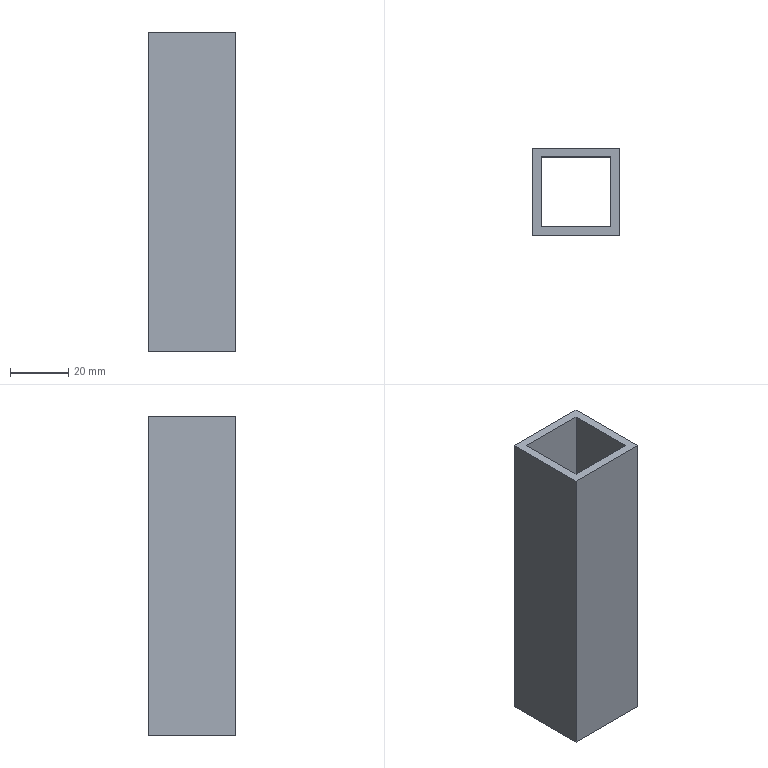Part | SolidWorks | features Cut 1, Extrusion 1 | 1 solid | 10 faces | box 30 x 30 x 110 mm | volume 35640 mm3 | plane 10
STEP:
#1=CARTESIAN_POINT('',(30.,0.,40.));
#2=VERTEX_POINT('',#1);
#3=CARTESIAN_POINT('',(0.,0.,40.));
#4=VERTEX_POINT('',#3);
#5=CARTESIAN_POINT('',(30.,0.,40.));
#6=DIRECTION('',(-1.,0.,0.));
#7=VECTOR('',#6,1000.);
#8=LINE('',#5,#7);
#9=EDGE_CURVE('',#2,#4,#8,.T.);
#10=ORIENTED_EDGE('',*,*,#9,.F.);
#11=CARTESIAN_POINT('',(30.,0.,150.));
#12=VERTEX_POINT('',#11);
#13=CARTESIAN_POINT('',(30.,0.,150.));
#14=DIRECTION('',(0.,0.,-1.));
#15=VECTOR('',#14,1000.);
#16=LINE('',#13,#15);
#17=EDGE_CURVE('',#12,#2,#16,.T.);
#18=ORIENTED_EDGE('',*,*,#17,.F.);
#19=CARTESIAN_POINT('',(0.,0.,150.));
#20=VERTEX_POINT('',#19);
#21=CARTESIAN_POINT('',(30.,0.,150.));
#22=DIRECTION('',(1.,0.,0.));
#23=VECTOR('',#22,1000.);
#24=LINE('',#21,#23);
#25=EDGE_CURVE('',#20,#12,#24,.T.);
#26=ORIENTED_EDGE('',*,*,#25,.F.);
#27=CARTESIAN_POINT('',(0.,0.,150.));
#28=DIRECTION('',(0.,0.,-1.));
#29=VECTOR('',#28,1000.);
#30=LINE('',#27,#29);
#31=EDGE_CURVE('',#20,#4,#30,.T.);
#32=ORIENTED_EDGE('',*,*,#31,.T.);
#33=EDGE_LOOP('',(#10,#18,#26,#32));
#34=FACE_OUTER_BOUND('',#33,.T.);
#35=CARTESIAN_POINT('',(30.,0.,150.));
#36=DIRECTION('',(0.,1.,0.));
#37=DIRECTION('',(0.,0.,1.));
#38=AXIS2_PLACEMENT_3D('',#35,#36,#37);
#39=PLANE('',#38);
#40=ADVANCED_FACE('',(#34),#39,.F.);
#41=CARTESIAN_POINT('',(30.,30.,40.));
#42=VERTEX_POINT('',#41);
#43=CARTESIAN_POINT('',(30.,30.,40.));
#44=DIRECTION('',(0.,-1.,0.));
#45=VECTOR('',#44,1000.);
#46=LINE('',#43,#45);
#47=EDGE_CURVE('',#42,#2,#46,.T.);
#48=ORIENTED_EDGE('',*,*,#47,.F.);
#49=CARTESIAN_POINT('',(30.,30.,150.));
#50=VERTEX_POINT('',#49);
#51=CARTESIAN_POINT('',(30.,30.,150.));
#52=DIRECTION('',(0.,0.,-1.));
#53=VECTOR('',#52,1000.);
#54=LINE('',#51,#53);
#55=EDGE_CURVE('',#50,#42,#54,.T.);
#56=ORIENTED_EDGE('',*,*,#55,.F.);
#57=CARTESIAN_POINT('',(30.,30.,150.));
#58=DIRECTION('',(0.,1.,0.));
#59=VECTOR('',#58,1000.);
#60=LINE('',#57,#59);
#61=EDGE_CURVE('',#12,#50,#60,.T.);
#62=ORIENTED_EDGE('',*,*,#61,.F.);
#63=ORIENTED_EDGE('',*,*,#17,.T.);
#64=EDGE_LOOP('',(#48,#56,#62,#63));
#65=FACE_OUTER_BOUND('',#64,.T.);
#66=CARTESIAN_POINT('',(30.,30.,150.));
#67=DIRECTION('',(-1.,0.,0.));
#68=DIRECTION('',(0.,0.,1.));
#69=AXIS2_PLACEMENT_3D('',#66,#67,#68);
#70=PLANE('',#69);
#71=ADVANCED_FACE('',(#65),#70,.F.);
#72=CARTESIAN_POINT('',(0.,30.,40.));
#73=VERTEX_POINT('',#72);
#74=CARTESIAN_POINT('',(0.,30.,40.));
#75=DIRECTION('',(1.,0.,0.));
#76=VECTOR('',#75,1000.);
#77=LINE('',#74,#76);
#78=EDGE_CURVE('',#73,#42,#77,.T.);
#79=ORIENTED_EDGE('',*,*,#78,.F.);
#80=CARTESIAN_POINT('',(0.,30.,150.));
#81=VERTEX_POINT('',#80);
#82=CARTESIAN_POINT('',(0.,30.,150.));
#83=DIRECTION('',(0.,0.,-1.));
#84=VECTOR('',#83,1000.);
#85=LINE('',#82,#84);
#86=EDGE_CURVE('',#81,#73,#85,.T.);
#87=ORIENTED_EDGE('',*,*,#86,.F.);
#88=CARTESIAN_POINT('',(0.,30.,150.));
#89=DIRECTION('',(-1.,0.,0.));
#90=VECTOR('',#89,1000.);
#91=LINE('',#88,#90);
#92=EDGE_CURVE('',#50,#81,#91,.T.);
#93=ORIENTED_EDGE('',*,*,#92,.F.);
#94=ORIENTED_EDGE('',*,*,#55,.T.);
#95=EDGE_LOOP('',(#79,#87,#93,#94));
#96=FACE_OUTER_BOUND('',#95,.T.);
#97=CARTESIAN_POINT('',(0.,30.,150.));
#98=DIRECTION('',(0.,-1.,0.));
#99=DIRECTION('',(0.,0.,-1.));
#100=AXIS2_PLACEMENT_3D('',#97,#98,#99);
#101=PLANE('',#100);
#102=ADVANCED_FACE('',(#96),#101,.F.);
#103=CARTESIAN_POINT('',(0.,0.,40.));
#104=DIRECTION('',(0.,1.,0.));
#105=VECTOR('',#104,1000.);
#106=LINE('',#103,#105);
#107=EDGE_CURVE('',#4,#73,#106,.T.);
#108=ORIENTED_EDGE('',*,*,#107,.F.);
#109=ORIENTED_EDGE('',*,*,#31,.F.);
#110=CARTESIAN_POINT('',(0.,0.,150.));
#111=DIRECTION('',(0.,-1.,0.));
#112=VECTOR('',#111,1000.);
#113=LINE('',#110,#112);
#114=EDGE_CURVE('',#81,#20,#113,.T.);
#115=ORIENTED_EDGE('',*,*,#114,.F.);
#116=ORIENTED_EDGE('',*,*,#86,.T.);
#117=EDGE_LOOP('',(#108,#109,#115,#116));
#118=FACE_OUTER_BOUND('',#117,.T.);
#119=CARTESIAN_POINT('',(0.,0.,150.));
#120=DIRECTION('',(1.,0.,0.));
#121=DIRECTION('',(0.,0.,-1.));
#122=AXIS2_PLACEMENT_3D('',#119,#120,#121);
#123=PLANE('',#122);
#124=ADVANCED_FACE('',(#118),#123,.F.);
#125=CARTESIAN_POINT('',(27.,3.,150.));
#126=VERTEX_POINT('',#125);
#127=CARTESIAN_POINT('',(27.,3.,40.));
#128=VERTEX_POINT('',#127);
#129=CARTESIAN_POINT('',(27.,3.,150.));
#130=DIRECTION('',(0.,0.,-1.));
#131=VECTOR('',#130,1000.);
#132=LINE('',#129,#131);
#133=EDGE_CURVE('',#126,#128,#132,.T.);
#134=ORIENTED_EDGE('',*,*,#133,.T.);
#135=CARTESIAN_POINT('',(3.,3.,40.));
#136=VERTEX_POINT('',#135);
#137=CARTESIAN_POINT('',(27.,3.,40.));
#138=DIRECTION('',(-1.,0.,0.));
#139=VECTOR('',#138,1000.);
#140=LINE('',#137,#139);
#141=EDGE_CURVE('',#128,#136,#140,.T.);
#142=ORIENTED_EDGE('',*,*,#141,.T.);
#143=CARTESIAN_POINT('',(3.,3.,150.));
#144=VERTEX_POINT('',#143);
#145=CARTESIAN_POINT('',(3.,3.,150.));
#146=DIRECTION('',(0.,0.,-1.));
#147=VECTOR('',#146,1000.);
#148=LINE('',#145,#147);
#149=EDGE_CURVE('',#144,#136,#148,.T.);
#150=ORIENTED_EDGE('',*,*,#149,.F.);
#151=CARTESIAN_POINT('',(27.,3.,150.));
#152=DIRECTION('',(1.,0.,0.));
#153=VECTOR('',#152,1000.);
#154=LINE('',#151,#153);
#155=EDGE_CURVE('',#144,#126,#154,.T.);
#156=ORIENTED_EDGE('',*,*,#155,.T.);
#157=EDGE_LOOP('',(#134,#142,#150,#156));
#158=FACE_OUTER_BOUND('',#157,.T.);
#159=CARTESIAN_POINT('',(27.,3.,150.));
#160=DIRECTION('',(0.,1.,0.));
#161=DIRECTION('',(0.,0.,1.));
#162=AXIS2_PLACEMENT_3D('',#159,#160,#161);
#163=PLANE('',#162);
#164=ADVANCED_FACE('',(#158),#163,.T.);
#165=CARTESIAN_POINT('',(27.,27.,150.));
#166=VERTEX_POINT('',#165);
#167=CARTESIAN_POINT('',(27.,27.,40.));
#168=VERTEX_POINT('',#167);
#169=CARTESIAN_POINT('',(27.,27.,150.));
#170=DIRECTION('',(0.,0.,-1.));
#171=VECTOR('',#170,1000.);
#172=LINE('',#169,#171);
#173=EDGE_CURVE('',#166,#168,#172,.T.);
#174=ORIENTED_EDGE('',*,*,#173,.T.);
#175=CARTESIAN_POINT('',(27.,27.,40.));
#176=DIRECTION('',(0.,-1.,0.));
#177=VECTOR('',#176,1000.);
#178=LINE('',#175,#177);
#179=EDGE_CURVE('',#168,#128,#178,.T.);
#180=ORIENTED_EDGE('',*,*,#179,.T.);
#181=ORIENTED_EDGE('',*,*,#133,.F.);
#182=CARTESIAN_POINT('',(27.,27.,150.));
#183=DIRECTION('',(0.,1.,0.));
#184=VECTOR('',#183,1000.);
#185=LINE('',#182,#184);
#186=EDGE_CURVE('',#126,#166,#185,.T.);
#187=ORIENTED_EDGE('',*,*,#186,.T.);
#188=EDGE_LOOP('',(#174,#180,#181,#187));
#189=FACE_OUTER_BOUND('',#188,.T.);
#190=CARTESIAN_POINT('',(27.,27.,150.));
#191=DIRECTION('',(-1.,0.,0.));
#192=DIRECTION('',(0.,0.,1.));
#193=AXIS2_PLACEMENT_3D('',#190,#191,#192);
#194=PLANE('',#193);
#195=ADVANCED_FACE('',(#189),#194,.T.);
#196=CARTESIAN_POINT('',(3.,27.,150.));
#197=VERTEX_POINT('',#196);
#198=CARTESIAN_POINT('',(3.,27.,40.));
#199=VERTEX_POINT('',#198);
#200=CARTESIAN_POINT('',(3.,27.,150.));
#201=DIRECTION('',(0.,0.,-1.));
#202=VECTOR('',#201,1000.);
#203=LINE('',#200,#202);
#204=EDGE_CURVE('',#197,#199,#203,.T.);
#205=ORIENTED_EDGE('',*,*,#204,.T.);
#206=CARTESIAN_POINT('',(3.,27.,40.));
#207=DIRECTION('',(1.,0.,0.));
#208=VECTOR('',#207,1000.);
#209=LINE('',#206,#208);
#210=EDGE_CURVE('',#199,#168,#209,.T.);
#211=ORIENTED_EDGE('',*,*,#210,.T.);
#212=ORIENTED_EDGE('',*,*,#173,.F.);
#213=CARTESIAN_POINT('',(3.,27.,150.));
#214=DIRECTION('',(-1.,0.,0.));
#215=VECTOR('',#214,1000.);
#216=LINE('',#213,#215);
#217=EDGE_CURVE('',#166,#197,#216,.T.);
#218=ORIENTED_EDGE('',*,*,#217,.T.);
#219=EDGE_LOOP('',(#205,#211,#212,#218));
#220=FACE_OUTER_BOUND('',#219,.T.);
#221=CARTESIAN_POINT('',(3.,27.,150.));
#222=DIRECTION('',(0.,-1.,0.));
#223=DIRECTION('',(0.,0.,-1.));
#224=AXIS2_PLACEMENT_3D('',#221,#222,#223);
#225=PLANE('',#224);
#226=ADVANCED_FACE('',(#220),#225,.T.);
#227=ORIENTED_EDGE('',*,*,#149,.T.);
#228=CARTESIAN_POINT('',(3.,3.,40.));
#229=DIRECTION('',(0.,1.,0.));
#230=VECTOR('',#229,1000.);
#231=LINE('',#228,#230);
#232=EDGE_CURVE('',#136,#199,#231,.T.);
#233=ORIENTED_EDGE('',*,*,#232,.T.);
#234=ORIENTED_EDGE('',*,*,#204,.F.);
#235=CARTESIAN_POINT('',(3.,3.,150.));
#236=DIRECTION('',(0.,-1.,0.));
#237=VECTOR('',#236,1000.);
#238=LINE('',#235,#237);
#239=EDGE_CURVE('',#197,#144,#238,.T.);
#240=ORIENTED_EDGE('',*,*,#239,.T.);
#241=EDGE_LOOP('',(#227,#233,#234,#240));
#242=FACE_OUTER_BOUND('',#241,.T.);
#243=CARTESIAN_POINT('',(3.,3.,150.));
#244=DIRECTION('',(1.,0.,0.));
#245=DIRECTION('',(0.,0.,-1.));
#246=AXIS2_PLACEMENT_3D('',#243,#244,#245);
#247=PLANE('',#246);
#248=ADVANCED_FACE('',(#242),#247,.T.);
#249=ORIENTED_EDGE('',*,*,#25,.T.);
#250=ORIENTED_EDGE('',*,*,#61,.T.);
#251=ORIENTED_EDGE('',*,*,#92,.T.);
#252=ORIENTED_EDGE('',*,*,#114,.T.);
#253=EDGE_LOOP('',(#249,#250,#251,#252));
#254=FACE_OUTER_BOUND('',#253,.T.);
#255=ORIENTED_EDGE('',*,*,#155,.F.);
#256=ORIENTED_EDGE('',*,*,#239,.F.);
#257=ORIENTED_EDGE('',*,*,#217,.F.);
#258=ORIENTED_EDGE('',*,*,#186,.F.);
#259=EDGE_LOOP('',(#255,#256,#257,#258));
#260=FACE_BOUND('',#259,.T.);
#261=CARTESIAN_POINT('',(0.,0.,150.));
#262=DIRECTION('',(0.,0.,-1.));
#263=DIRECTION('',(-1.,0.,0.));
#264=AXIS2_PLACEMENT_3D('',#261,#262,#263);
#265=PLANE('',#264);
#266=ADVANCED_FACE('',(#254,#260),#265,.F.);
#267=ORIENTED_EDGE('',*,*,#179,.F.);
#268=ORIENTED_EDGE('',*,*,#210,.F.);
#269=ORIENTED_EDGE('',*,*,#232,.F.);
#270=ORIENTED_EDGE('',*,*,#141,.F.);
#271=EDGE_LOOP('',(#267,#268,#269,#270));
#272=FACE_BOUND('',#271,.T.);
#273=ORIENTED_EDGE('',*,*,#47,.T.);
#274=ORIENTED_EDGE('',*,*,#9,.T.);
#275=ORIENTED_EDGE('',*,*,#107,.T.);
#276=ORIENTED_EDGE('',*,*,#78,.T.);
#277=EDGE_LOOP('',(#273,#274,#275,#276));
#278=FACE_OUTER_BOUND('',#277,.T.);
#279=CARTESIAN_POINT('',(0.,0.,40.));
#280=DIRECTION('',(0.,0.,-1.));
#281=DIRECTION('',(-1.,0.,0.));
#282=AXIS2_PLACEMENT_3D('',#279,#280,#281);
#283=PLANE('',#282);
#284=ADVANCED_FACE('',(#272,#278),#283,.T.);
#285=CLOSED_SHELL('',(#40,#71,#102,#124,#164,#195,#226,#248,#266,#284));
#286=MANIFOLD_SOLID_BREP('',#285);
#287=CARTESIAN_POINT('',(0.,0.,0.));
#288=DIRECTION('',(0.,0.,1.));
#289=DIRECTION('',(1.,0.,0.));
#290=AXIS2_PLACEMENT_3D('',#287,#288,#289);
#291=(LENGTH_UNIT()NAMED_UNIT(*)SI_UNIT(.MILLI.,.METRE.));
#292=UNCERTAINTY_MEASURE_WITH_UNIT(LENGTH_MEASURE(0.00001),#291,'','');
#293=(NAMED_UNIT(*)PLANE_ANGLE_UNIT()SI_UNIT($,.RADIAN.));
#294=(NAMED_UNIT(*)SI_UNIT($,.STERADIAN.)SOLID_ANGLE_UNIT());
#295=(GEOMETRIC_REPRESENTATION_CONTEXT(3)GLOBAL_UNCERTAINTY_ASSIGNED_CONTEXT((#292))GLOBAL_UNIT_ASSIGNED_CONTEXT((#291,#293,#294))REPRESENTATION_CONTEXT('',''));
#296=ADVANCED_BREP_SHAPE_REPRESENTATION('',(#286,#290),#295);